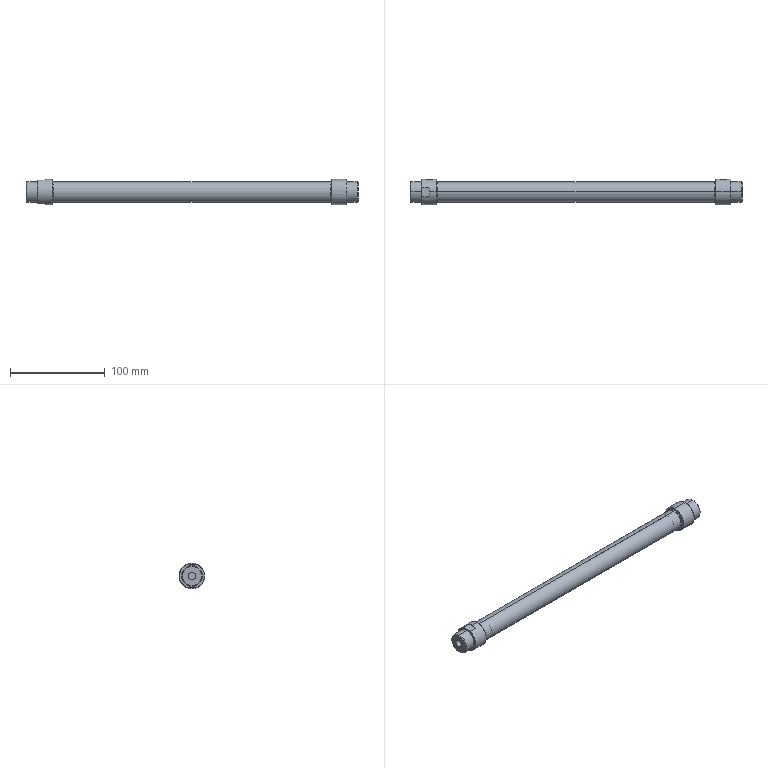Part | SolidWorks | features BaseBody 1 | 1 solid | 59 faces | box 350 x 27 x 27 mm | volume 44687 mm3 | cylinder 22 | plane 16 | cone 13 | spline 8 | commonest cylinder face diameters 21.4 x6 8.566 x4 22 x4 27 x4 8 x2 20 x2